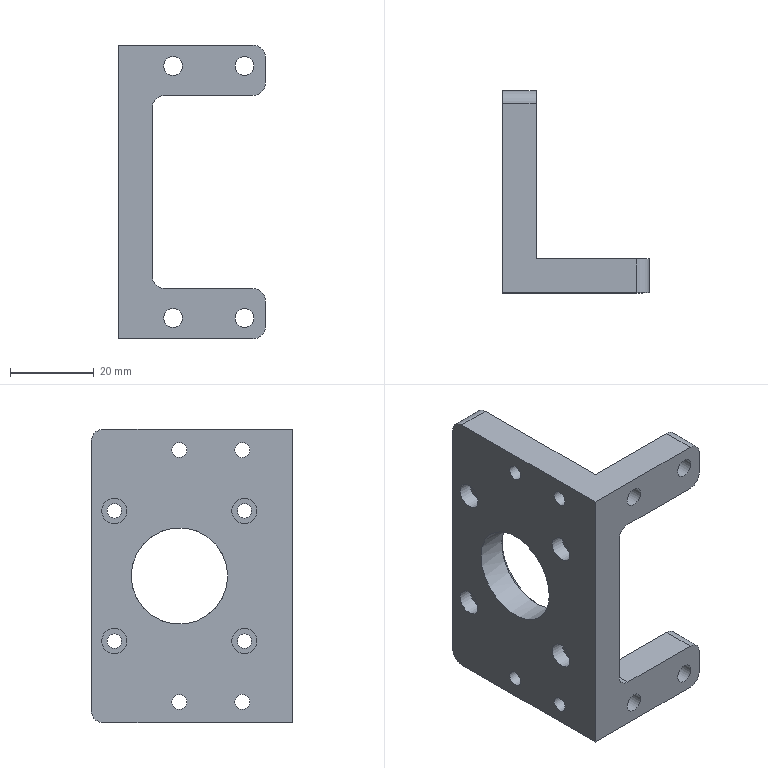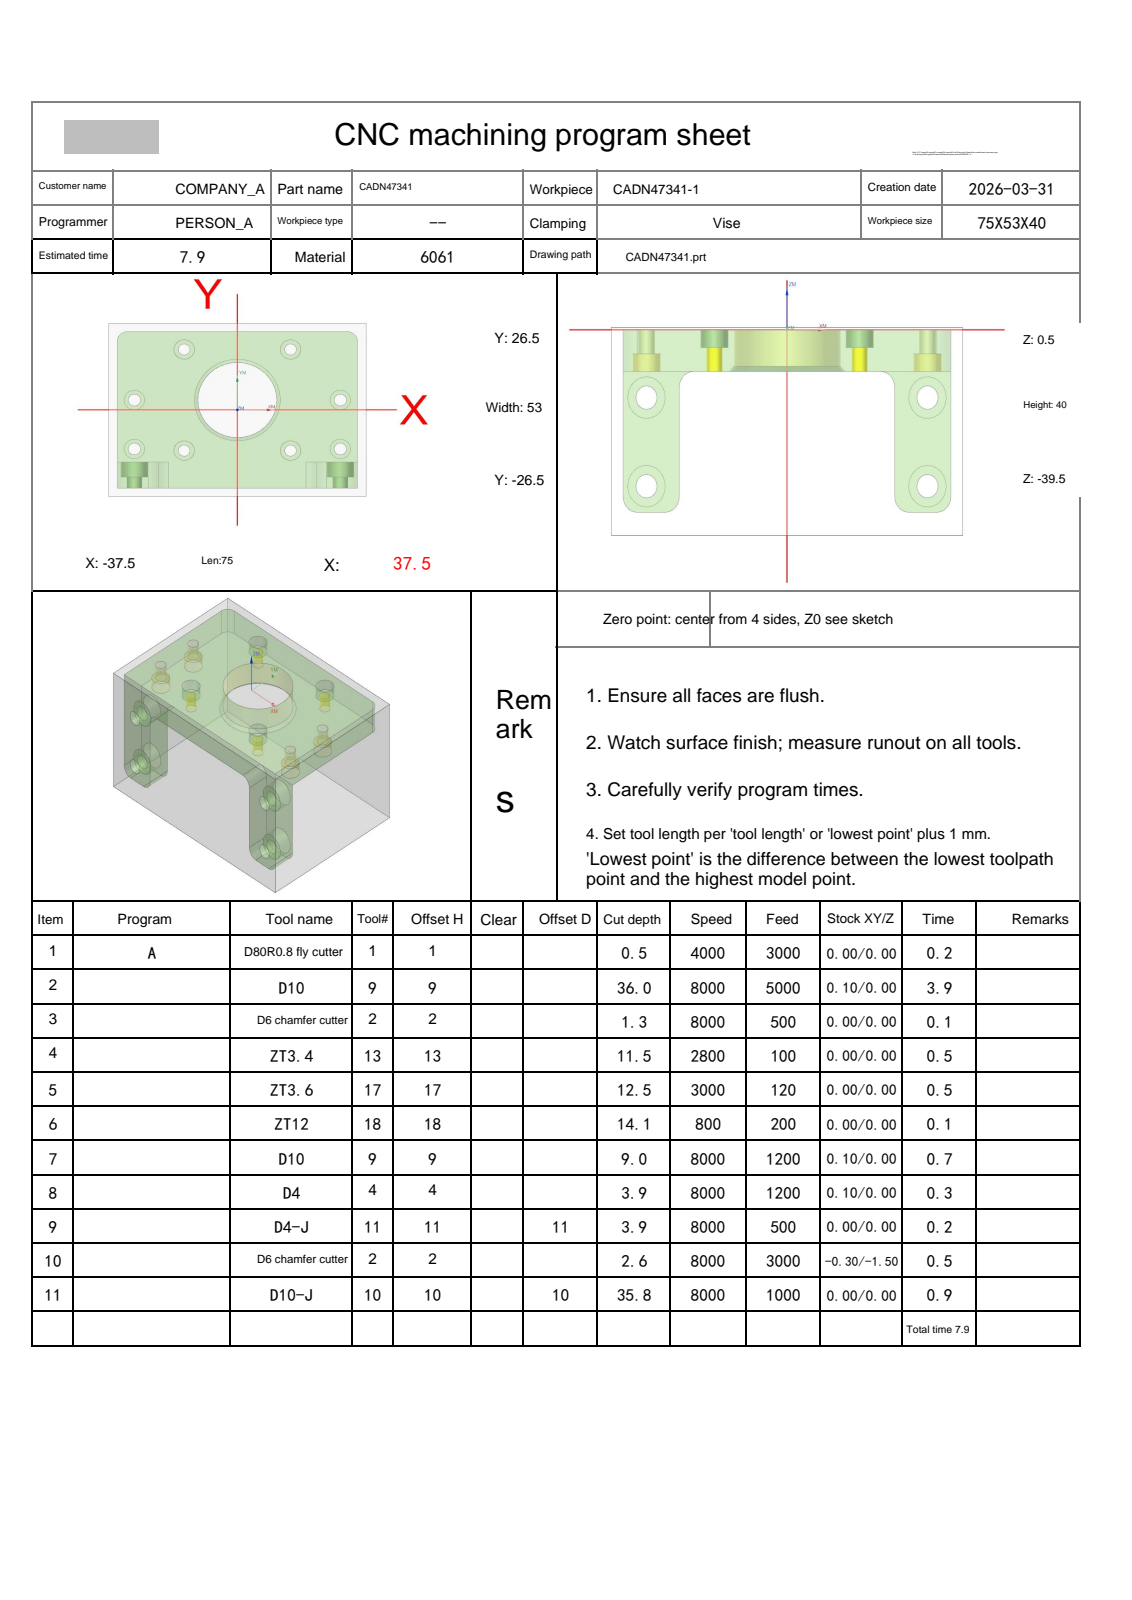NC program | NX | posted by the shop | part box 35 x 48 x 70 mm
Whole program:
%
O0001
(Machine time: 9.90 MIN)
(===Total Tool:9===)
(T1=D80R0.8 fly cutter D=80.  R=0.8  D-  H01 Z=0.    )
(T9=D10     D=10.  R=0.   D-  H09 Z=-35.5 )
(T2=D6 chamfer cutter   D=6.   R=0.   D-  H02 Z=-2.1  )
(T13=ZT3.4  D=3.4  DR_a=118 D-  H13 Z=-11.02)
(T17=ZT3.6  D=3.6  DR_a=118 D-  H17 Z=-12.  )
(T18=ZT12   D=12.  DR_a=118 D-  H18 Z=-13.61)
(T4=D4      D=4.   R=0.   D-  H04 Z=-3.4  )
(T11=D4-J   D=4.   R=0.   D11 H11 Z=-3.4  )
(T10=D10-J  D=10.  R=0.   D10 H10 Z=-35.3 )
G80 G90 G17 G49 G40
G91 G28 Z0
M01
N1 T01 M06
(D80R0.8 fly cutter  D=80. R=0.8 H=01 ce=0.20 di=0.10)
G00 G90 G54 X-80. Y0.0 M03 S4000
G43 H01 Z20.
M08
Z2.1
G01 Z.1 F3000.
X-75.
X75.
X80.
Z2.1
G00 Z20.
G00 G90 X-80. Y0.0 M03 S4000
Z20.
Z2.
G01 Z0.0 F1000.
X-75.
X75.
X80.
Z2.
G00 Z20.
G91 G28 Z0.0
M05
M09
G91 G28 Z0.0
M01
N2 T09 M06
(D10  D=10. R=0. H=09 ce=0.10 di=0.00)
G00 G90 G54 X0.0 Y-29.1 M03 S8000
G43 H09 Z20.
M08
Z.5
G01 X-35. Z.435 F5000.
G02 X-40.1 Y-24. Z.42 I0.0 J5.1
G01 Y21. Z.337
G02 X-32. Y29.1 Z.313 I8.1 J0.0
G01 X32. Z.194
G02 X40.1 Y21. Z.17 I0.0 J-8.1
G01 Y-24. Z.087
G02 X35. Y-29.1 Z.072 I-5.1 J0.0
G01 X-35. Z-.058
G02 X-40.1 Y-24. Z-.073 I0.0 J5.1
G01 Y21. Z-.157
G02 X-32. Y29.1 Z-.18 I8.1 J0.0
G01 X32. Z-.299
G02 X40.1 Y21. Z-.323 I0.0 J-8.1
G01 Y-24. Z-.406
G02 X35. Y-29.1 Z-.421 I-5.1 J0.0
G01 X-35. Z-.551
G02 X-40.1 Y-24. Z-.566 I0.0 J5.1
G01 Y21. Z-.65
G02 X-32. Y29.1 Z-.673 I8.1 J0.0
G01 X32. Z-.792
G02 X40.1 Y21. Z-.816 I0.0 J-8.1
G01 Y-24. Z-.9
G02 X35. Y-29.1 Z-.914 I-5.1 J0.0
G01 X-35. Z-1.044
G02 X-40.1 Y-24. Z-1.059 I0.0 J5.1
G01 Y21. Z-1.143
G02 X-32. Y29.1 Z-1.167 I8.1 J0.0
G01 X32. Z-1.285
G02 X40.1 Y21. Z-1.309 I0.0 J-8.1
G01 Y-24. Z-1.393
G02 X35. Y-29.1 Z-1.408 I-5.1 J0.0
G01 X-35. Z-1.538
G02 X-40.1 Y-24. Z-1.553 I0.0 J5.1
G01 Y21. Z-1.636
G02 X-32. Y29.1 Z-1.66 I8.1 J0.0
G01 X32. Z-1.779
G02 X40.1 Y21. Z-1.802 I0.0 J-8.1
G01 Y-24. Z-1.886
G02 X35. Y-29.1 Z-1.901 I-5.1 J0.0
G01 X-35. Z-2.031
G02 X-40.1 Y-24. Z-2.046 I0.0 J5.1
G01 Y21. Z-2.129
G02 X-32. Y29.1 Z-2.153 I8.1 J0.0
G01 X32. Z-2.272
G02 X40.1 Y21. Z-2.295 I0.0 J-8.1
G01 Y-24. Z-2.379
G02 X35. Y-29.1 Z-2.394 I-5.1 J0.0
G01 X-35. Z-2.524
G02 X-40.1 Y-24. Z-2.539 I0.0 J5.1
G01 Y21. Z-2.622
G02 X-32. Y29.1 Z-2.646 I8.1 J0.0
G01 X32. Z-2.765
G02 X40.1 Y21. Z-2.789 I0.0 J-8.1
G01 Y-24. Z-2.872
G02 X35. Y-29.1 Z-2.887 I-5.1 J0.0
G01 X-35. Z-3.017
G02 X-40.1 Y-24. Z-3.032 I0.0 J5.1
G01 Y21. Z-3.116
G02 X-32. Y29.1 Z-3.139 I8.1 J0.0
G01 X32. Z-3.258
G02 X40.1 Y21. Z-3.282 I0.0 J-8.1
G01 Y-24. Z-3.365
G02 X35. Y-29.1 Z-3.38 I-5.1 J0.0
G01 X-35. Z-3.51
G02 X-40.1 Y-24. Z-3.525 I0.0 J5.1
G01 Y21. Z-3.609
G02 X-32. Y29.1 Z-3.632 I8.1 J0.0
G01 X32. Z-3.751
G02 X40.1 Y21. Z-3.775 I0.0 J-8.1
G01 Y-24. Z-3.858
G02 X35. Y-29.1 Z-3.873 I-5.1 J0.0
G01 X-35. Z-4.003
G02 X-40.1 Y-24. Z-4.018 I0.0 J5.1
G01 Y21. Z-4.102
G02 X-32. Y29.1 Z-4.125 I8.1 J0.0
G01 X32. Z-4.244
G02 X40.1 Y21. Z-4.268 I0.0 J-8.1
G01 Y-24. Z-4.352
G02 X35. Y-29.1 Z-4.366 I-5.1 J0.0
G01 X-35. Z-4.497
G02 X-40.1 Y-24. Z-4.511 I0.0 J5.1
G01 Y21. Z-4.595
G02 X-32. Y29.1 Z-4.619 I8.1 J0.0
G01 X32. Z-4.738
G02 X40.1 Y21. Z-4.761 I0.0 J-8.1
G01 Y-24. Z-4.845
G02 X35. Y-29.1 Z-4.86 I-5.1 J0.0
G01 X-35. Z-4.99
G02 X-40.1 Y-24. Z-5.005 I0.0 J5.1
G01 Y21. Z-5.088
G02 X-32. Y29.1 Z-5.112 I8.1 J0.0
G01 X32. Z-5.231
G02 X40.1 Y21. Z-5.254 I0.0 J-8.1
G01 Y-24. Z-5.338
G02 X35. Y-29.1 Z-5.353 I-5.1 J0.0
G01 X-35. Z-5.483
G02 X-40.1 Y-24. Z-5.498 I0.0 J5.1
G01 Y21. Z-5.581
G02 X-32. Y29.1 Z-5.605 I8.1 J0.0
G01 X32. Z-5.724
G02 X40.1 Y21. Z-5.747 I0.0 J-8.1
G01 Y-24. Z-5.831
G02 X35. Y-29.1 Z-5.846 I-5.1 J0.0
G01 X-35. Z-5.976
G02 X-40.1 Y-24. Z-5.991 I0.0 J5.1
G01 Y21. Z-6.074
G02 X-32. Y29.1 Z-6.098 I8.1 J0.0
G01 X32. Z-6.217
G02 X40.1 Y21. Z-6.241 I0.0 J-8.1
G01 Y-24. Z-6.324
G02 X35. Y-29.1 Z-6.339 I-5.1 J0.0
G01 X-35. Z-6.469
G02 X-40.1 Y-24. Z-6.484 I0.0 J5.1
G01 Y21. Z-6.568
G02 X-32. Y29.1 Z-6.591 I8.1 J0.0
G01 X32. Z-6.71
G02 X40.1 Y21. Z-6.734 I0.0 J-8.1
G01 Y-24. Z-6.817
G02 X35. Y-29.1 Z-6.832 I-5.1 J0.0
G01 X-35. Z-6.962
G02 X-40.1 Y-24. Z-6.977 I0.0 J5.1
G01 Y21. Z-7.061
G02 X-32. Y29.1 Z-7.084 I8.1 J0.0
G01 X32. Z-7.203
G02 X40.1 Y21. Z-7.227 I0.0 J-8.1
G01 Y-24. Z-7.311
G02 X35. Y-29.1 Z-7.325 I-5.1 J0.0
G01 X-35. Z-7.455
G02 X-40.1 Y-24. Z-7.47 I0.0 J5.1
G01 Y21. Z-7.554
G02 X-32. Y29.1 Z-7.578 I8.1 J0.0
G01 X32. Z-7.696
G02 X40.1 Y21. Z-7.72 I0.0 J-8.1
G01 Y-24. Z-7.804
G02 X35. Y-29.1 Z-7.819 I-5.1 J0.0
G01 X-35. Z-7.949
G02 X-40.1 Y-24. Z-7.963 I0.0 J5.1
G01 Y21. Z-8.047
G02 X-32. Y29.1 Z-8.071 I8.1 J0.0
G01 X32. Z-8.19
G02 X40.1 Y21. Z-8.213 I0.0 J-8.1
G01 Y-24. Z-8.297
G02 X35. Y-29.1 Z-8.312 I-5.1 J0.0
G01 X-35. Z-8.442
G02 X-40.1 Y-24. Z-8.457 I0.0 J5.1
G01 Y21. Z-8.54
G02 X-32. Y29.1 Z-8.564 I8.1 J0.0
G01 X32. Z-8.683
G02 X40.1 Y21. Z-8.706 I0.0 J-8.1
G01 Y-24. Z-8.79
G02 X35. Y-29.1 Z-8.805 I-5.1 J0.0
G01 X-35. Z-8.935
G02 X-40.1 Y-24. Z-8.95 I0.0 J5.1
G01 Y21. Z-9.033
G02 X-32. Y29.1 Z-9.057 I8.1 J0.0
G01 X32. Z-9.176
G02 X40.1 Y21. Z-9.2 I0.0 J-8.1
G01 Y-24. Z-9.283
G02 X35. Y-29.1 Z-9.298 I-5.1 J0.0
G01 X-35. Z-9.428
G02 X-40.1 Y-24. Z-9.443 I0.0 J5.1
G01 Y21. Z-9.527
G02 X-32. Y29.1 Z-9.55 I8.1 J0.0
G01 X32. Z-9.669
G02 X40.1 Y21. Z-9.693 I0.0 J-8.1
G01 Y-24. Z-9.776
G02 X35. Y-29.1 Z-9.791 I-5.1 J0.0
G01 X-35. Z-9.921
G02 X-40.1 Y-24. Z-9.936 I0.0 J5.1
G01 Y21. Z-10.02
G02 X-32. Y29.1 Z-10.043 I8.1 J0.0
G01 X32. Z-10.162
G02 X40.1 Y21. Z-10.186 I0.0 J-8.1
G01 Y-24. Z-10.269
G02 X35. Y-29.1 Z-10.284 I-5.1 J0.0
G01 X-35. Z-10.414
G02 X-40.1 Y-24. Z-10.429 I0.0 J5.1
G01 Y21. Z-10.513
G02 X-32. Y29.1 Z-10.536 I8.1 J0.0
G01 X32. Z-10.655
G02 X40.1 Y21. Z-10.679 I0.0 J-8.1
G01 Y-24. Z-10.763
G02 X35. Y-29.1 Z-10.777 I-5.1 J0.0
G01 X-35. Z-10.907
G02 X-40.1 Y-24. Z-10.922 I0.0 J5.1
G01 Y21. Z-11.006
G02 X-32. Y29.1 Z-11.03 I8.1 J0.0
G01 X32. Z-11.148
G02 X40.1 Y21. Z-11.172 I0.0 J-8.1
G01 Y-24. Z-11.256
G02 X35. Y-29.1 Z-11.271 I-5.1 J0.0
G01 X-35. Z-11.401
G02 X-40.1 Y-24. Z-11.416 I0.0 J5.1
G01 Y21. Z-11.499
G02 X-32. Y29.1 Z-11.523 I8.1 J0.0
G01 X32. Z-11.642
G02 X40.1 Y21. Z-11.665 I0.0 J-8.1
G01 Y-24. Z-11.749
G02 X35. Y-29.1 Z-11.764 I-5.1 J0.0
G01 X-35. Z-11.894
G02 X-40.1 Y-24. Z-11.909 I0.0 J5.1
G01 Y21. Z-11.992
G02 X-32. Y29.1 Z-12.016 I8.1 J0.0
G01 X32. Z-12.135
G02 X40.1 Y21. Z-12.158 I0.0 J-8.1
G01 Y-24. Z-12.242
G02 X35. Y-29.1 Z-12.257 I-5.1 J0.0
G01 X-35. Z-12.387
G02 X-40.1 Y-24. Z-12.402 I0.0 J5.1
G01 Y21. Z-12.485
G02 X-32. Y29.1 Z-12.509 I8.1 J0.0
G01 X32. Z-12.628
G02 X40.1 Y21. Z-12.652 I0.0 J-8.1
G01 Y-24. Z-12.735
G02 X35. Y-29.1 Z-12.75 I-5.1 J0.0
G01 X-35. Z-12.88
G02 X-40.1 Y-24. Z-12.895 I0.0 J5.1
G01 Y21. Z-12.979
G02 X-32. Y29.1 Z-13.002 I8.1 J0.0
G01 X32. Z-13.121
G02 X40.1 Y21. Z-13.145 I0.0 J-8.1
G01 Y-24. Z-13.228
G02 X35. Y-29.1 Z-13.243 I-5.1 J0.0
G01 X-35. Z-13.373
G02 X-40.1 Y-24. Z-13.388 I0.0 J5.1
G01 Y21. Z-13.472
G02 X-32. Y29.1 Z-13.495 I8.1 J0.0
G01 X32. Z-13.614
G02 X40.1 Y21. Z-13.638 I0.0 J-8.1
G01 Y-24. Z-13.721
G02 X35. Y-29.1 Z-13.736 I-5.1 J0.0
G01 X-35. Z-13.866
G02 X-40.1 Y-24. Z-13.881 I0.0 J5.1
G01 Y21. Z-13.965
G02 X-32. Y29.1 Z-13.989 I8.1 J0.0
G01 X32. Z-14.107
G02 X40.1 Y21. Z-14.131 I0.0 J-8.1
G01 Y-24. Z-14.215
G02 X35. Y-29.1 Z-14.23 I-5.1 J0.0
G01 X-35. Z-14.36
G02 X-40.1 Y-24. Z-14.374 I0.0 J5.1
G01 Y21. Z-14.458
G02 X-32. Y29.1 Z-14.482 I8.1 J0.0
G01 X32. Z-14.601
G02 X40.1 Y21. Z-14.624 I0.0 J-8.1
G01 Y-24. Z-14.708
G02 X35. Y-29.1 Z-14.723 I-5.1 J0.0
G01 X-35. Z-14.853
G02 X-40.1 Y-24. Z-14.868 I0.0 J5.1
G01 Y21. Z-14.951
G02 X-32. Y29.1 Z-14.975 I8.1 J0.0
G01 X32. Z-15.094
G02 X40.1 Y21. Z-15.117 I0.0 J-8.1
G01 Y-24. Z-15.201
G02 X35. Y-29.1 Z-15.216 I-5.1 J0.0
G01 X-35. Z-15.346
G02 X-40.1 Y-24. Z-15.361 I0.0 J5.1
G01 Y21. Z-15.444
G02 X-32. Y29.1 Z-15.468 I8.1 J0.0
G01 X32. Z-15.587
G02 X40.1 Y21. Z-15.61 I0.0 J-8.1
G01 Y-24. Z-15.694
G02 X35. Y-29.1 Z-15.709 I-5.1 J0.0
G01 X-35. Z-15.839
G02 X-40.1 Y-24. Z-15.854 I0.0 J5.1
G01 Y21. Z-15.937
G02 X-32. Y29.1 Z-15.961 I8.1 J0.0
G01 X32. Z-16.08
G02 X40.1 Y21. Z-16.104 I0.0 J-8.1
G01 Y-24. Z-16.187
G02 X35. Y-29.1 Z-16.202 I-5.1 J0.0
G01 X-35. Z-16.332
G02 X-40.1 Y-24. Z-16.347 I0.0 J5.1
G01 Y21. Z-16.431
G02 X-32. Y29.1 Z-16.454 I8.1 J0.0
G01 X32. Z-16.573
G02 X40.1 Y21. Z-16.597 I0.0 J-8.1
G01 Y-24. Z-16.68
G02 X35. Y-29.1 Z-16.695 I-5.1 J0.0
G01 X-35. Z-16.825
G02 X-40.1 Y-24. Z-16.84 I0.0 J5.1
G01 Y21. Z-16.924
G02 X-32. Y29.1 Z-16.947 I8.1 J0.0
G01 X32. Z-17.066
G02 X40.1 Y21. Z-17.09 I0.0 J-8.1
G01 Y-24. Z-17.174
G02 X35. Y-29.1 Z-17.188 I-5.1 J0.0
G01 X-35. Z-17.318
G02 X-40.1 Y-24. Z-17.333 I0.0 J5.1
G01 Y21. Z-17.417
G02 X-32. Y29.1 Z-17.441 I8.1 J0.0
G01 X32. Z-17.559
G02 X40.1 Y21. Z-17.583 I0.0 J-8.1
G01 Y-24. Z-17.667
G02 X35. Y-29.1 Z-17.682 I-5.1 J0.0
G01 X-35. Z-17.812
G02 X-40.1 Y-24. Z-17.826 I0.0 J5.1
G01 Y21. Z-17.91
G02 X-32. Y29.1 Z-17.934 I8.1 J0.0
G01 X32. Z-18.053
G02 X40.1 Y21. Z-18.076 I0.0 J-8.1
G01 Y-24. Z-18.16
G02 X35. Y-29.1 Z-18.175 I-5.1 J0.0
G01 X-35. Z-18.305
G02 X-40.1 Y-24. Z-18.32 I0.0 J5.1
G01 Y21. Z-18.403
G02 X-32. Y29.1 Z-18.427 I8.1 J0.0
G01 X32. Z-18.546
G02 X40.1 Y21. Z-18.569 I0.0 J-8.1
G01 Y-24. Z-18.653
G02 X35. Y-29.1 Z-18.668 I-5.1 J0.0
G01 X-35. Z-18.798
G02 X-40.1 Y-24. Z-18.813 I0.0 J5.1
G01 Y21. Z-18.896
G02 X-32. Y29.1 Z-18.92 I8.1 J0.0
G01 X32. Z-19.039
G02 X40.1 Y21. Z-19.063 I0.0 J-8.1
G01 Y-24. Z-19.146
G02 X35. Y-29.1 Z-19.161 I-5.1 J0.0
G01 X-35. Z-19.291
G02 X-40.1 Y-24. Z-19.306 I0.0 J5.1
G01 Y21. Z-19.39
G02 X-32. Y29.1 Z-19.413 I8.1 J0.0
G01 X32. Z-19.532
G02 X40.1 Y21. Z-19.556 I0.0 J-8.1
G01 Y-24. Z-19.639
G02 X35. Y-29.1 Z-19.654 I-5.1 J0.0
G01 X-35. Z-19.784
G02 X-40.1 Y-24. Z-19.799 I0.0 J5.1
G01 Y21. Z-19.883
G02 X-32. Y29.1 Z-19.906 I8.1 J0.0
G01 X32. Z-20.025
G02 X40.1 Y21. Z-20.049 I0.0 J-8.1
G01 Y-24. Z-20.132
G02 X35. Y-29.1 Z-20.147 I-5.1 J0.0
G01 X-35. Z-20.277
G02 X-40.1 Y-24. Z-20.292 I0.0 J5.1
G01 Y21. Z-20.376
G02 X-32. Y29.1 Z-20.399 I8.1 J0.0
G01 X32. Z-20.518
G02 X40.1 Y21. Z-20.542 I0.0 J-8.1
G01 Y-24. Z-20.626
G02 X35. Y-29.1 Z-20.64 I-5.1 J0.0
G01 X-35. Z-20.77
G02 X-40.1 Y-24. Z-20.785 I0.0 J5.1
G01 Y21. Z-20.869
G02 X-32. Y29.1 Z-20.893 I8.1 J0.0
G01 X32. Z-21.012
G02 X40.1 Y21. Z-21.035 I0.0 J-8.1
G01 Y-24. Z-21.119
G02 X35. Y-29.1 Z-21.134 I-5.1 J0.0
G01 X-35. Z-21.264
G02 X-40.1 Y-24. Z-21.279 I0.0 J5.1
G01 Y21. Z-21.362
G02 X-32. Y29.1 Z-21.386 I8.1 J0.0
G01 X32. Z-21.505
G02 X40.1 Y21. Z-21.528 I0.0 J-8.1
G01 Y-24. Z-21.612
G02 X35. Y-29.1 Z-21.627 I-5.1 J0.0
G01 X-35. Z-21.757
G02 X-40.1 Y-24. Z-21.772 I0.0 J5.1
G01 Y21. Z-21.855
G02 X-32. Y29.1 Z-21.879 I8.1 J0.0
G01 X32. Z-21.998
G02 X40.1 Y21. Z-22.021 I0.0 J-8.1
G01 Y-24. Z-22.105
G02 X35. Y-29.1 Z-22.12 I-5.1 J0.0
G01 X-35. Z-22.25
G02 X-40.1 Y-24. Z-22.265 I0.0 J5.1
G01 Y21. Z-22.348
G02 X-32. Y29.1 Z-22.372 I8.1 J0.0
G01 X32. Z-22.491
G02 X40.1 Y21. Z-22.515 I0.0 J-8.1
G01 Y-24. Z-22.598
G02 X35. Y-29.1 Z-22.613 I-5.1 J0.0
G01 X-35. Z-22.743
G02 X-40.1 Y-24. Z-22.758 I0.0 J5.1
G01 Y21. Z-22.842
G02 X-32. Y29.1 Z-22.865 I8.1 J0.0
G01 X32. Z-22.984
G02 X40.1 Y21. Z-23.008 I0.0 J-8.1
G01 Y-24. Z-23.091
G02 X35. Y-29.1 Z-23.106 I-5.1 J0.0
G01 X-35. Z-23.236
G02 X-40.1 Y-24. Z-23.251 I0.0 J5.1
G01 Y21. Z-23.335
G02 X-32. Y29.1 Z-23.358 I8.1 J0.0
G01 X32. Z-23.477
G02 X40.1 Y21. Z-23.501 I0.0 J-8.1
G01 Y-24. Z-23.584
G02 X35. Y-29.1 Z-23.599 I-5.1 J0.0
G01 X-35. Z-23.729
G02 X-40.1 Y-24. Z-23.744 I0.0 J5.1
G01 Y21. Z-23.828
G02 X-32. Y29.1 Z-23.852 I8.1 J0.0
G01 X32. Z-23.97
G02 X40.1 Y21. Z-23.994 I0.0 J-8.1
G01 Y-24. Z-24.078
G02 X35. Y-29.1 Z-24.093 I-5.1 J0.0
G01 X-35. Z-24.223
G02 X-40.1 Y-24. Z-24.237 I0.0 J5.1
G01 Y21. Z-24.321
G02 X-32. Y29.1 Z-24.345 I8.1 J0.0
G01 X32. Z-24.464
G02 X40.1 Y21. Z-24.487 I0.0 J-8.1
G01 Y-24. Z-24.571
G02 X35. Y-29.1 Z-24.586 I-5.1 J0.0
G01 X-35. Z-24.716
G02 X-40.1 Y-24. Z-24.731 I0.0 J5.1
G01 Y21. Z-24.814
G02 X-32. Y29.1 Z-24.838 I8.1 J0.0
G01 X32. Z-24.957
G02 X40.1 Y21. Z-24.98 I0.0 J-8.1
G01 Y-24. Z-25.064
G02 X35. Y-29.1 Z-25.079 I-5.1 J0.0
G01 X-35. Z-25.209
G02 X-40.1 Y-24. Z-25.224 I0.0 J5.1
G01 Y21. Z-25.307
G02 X-32. Y29.1 Z-25.331 I8.1 J0.0
G01 X32. Z-25.45
G02 X40.1 Y21. Z-25.473 I0.0 J-8.1
G01 Y-24. Z-25.557
G02 X35. Y-29.1 Z-25.572 I-5.1 J0.0
G01 X-35. Z-25.702
G02 X-40.1 Y-24. Z-25.717 I0.0 J5.1
G01 Y21. Z-25.8
G02 X-32. Y29.1 Z-25.824 I8.1 J0.0
G01 X32. Z-25.943
G02 X40.1 Y21. Z-25.967 I0.0 J-8.1
G01 Y-24. Z-26.05
G02 X35. Y-29.1 Z-26.065 I-5.1 J0.0
G01 X-35. Z-26.195
G02 X-40.1 Y-24. Z-26.21 I0.0 J5.1
G01 Y21. Z-26.294
G02 X-32. Y29.1 Z-26.317 I8.1 J0.0
G01 X32. Z-26.436
G02 X40.1 Y21. Z-26.46 I0.0 J-8.1
G01 Y-24. Z-26.543
G02 X35. Y-29.1 Z-26.558 I-5.1 J0.0
G01 X-35. Z-26.688
G02 X-40.1 Y-24. Z-26.703 I0.0 J5.1
G01 Y21. Z-26.787
G02 X-32. Y29.1 Z-26.81 I8.1 J0.0
G01 X32. Z-26.929
G02 X40.1 Y21. Z-26.953 I0.0 J-8.1
G01 Y-24. Z-27.037
G02 X35. Y-29.1 Z-27.051 I-5.1 J0.0
G01 X-35. Z-27.181
G02 X-40.1 Y-24. Z-27.196 I0.0 J5.1
G01 Y21. Z-27.28
G02 X-32. Y29.1 Z-27.304 I8.1 J0.0
G01 X32. Z-27.422
G02 X40.1 Y21. Z-27.446 I0.0 J-8.1
G01 Y-24. Z-27.53
G02 X35. Y-29.1 Z-27.545 I-5.1 J0.0
G01 X-35. Z-27.675
G02 X-40.1 Y-24. Z-27.689 I0.0 J5.1
G01 Y21. Z-27.773
G02 X-32. Y29.1 Z-27.797 I8.1 J0.0
G01 X32. Z-27.916
G02 X40.1 Y21. Z-27.939 I0.0 J-8.1
G01 Y-24. Z-28.023
G02 X35. Y-29.1 Z-28.038 I-5.1 J0.0
G01 X-35. Z-28.168
G02 X-40.1 Y-24. Z-28.183 I0.0 J5.1
G01 Y21. Z-28.266
G02 X-32. Y29.1 Z-28.29 I8.1 J0.0
G01 X32. Z-28.409
G02 X40.1 Y21. Z-28.432 I0.0 J-8.1
G01 Y-24. Z-28.516
G02 X35. Y-29.1 Z-28.531 I-5.1 J0.0
G01 X-35. Z-28.661
G02 X-40.1 Y-24. Z-28.676 I0.0 J5.1
G01 Y21. Z-28.759
G02 X-32. Y29.1 Z-28.783 I8.1 J0.0
G01 X32. Z-28.902
G02 X40.1 Y21. Z-28.926 I0.0 J-8.1
G01 Y-24. Z-29.009
G02 X35. Y-29.1 Z-29.024 I-5.1 J0.0
G01 X-35. Z-29.154
G02 X-40.1 Y-24. Z-29.169 I0.0 J5.1
G01 Y21. Z-29.253
G02 X-32. Y29.1 Z-29.276 I8.1 J0.0
G01 X32. Z-29.395
G02 X40.1 Y21. Z-29.419 I0.0 J-8.1
G01 Y-24. Z-29.502
G02 X35. Y-29.1 Z-29.517 I-5.1 J0.0
G01 X-35. Z-29.647
G02 X-40.1 Y-24. Z-29.662 I0.0 J5.1
G01 Y21. Z-29.746
G02 X-32. Y29.1 Z-29.769 I8.1 J0.0
G01 X32. Z-29.888
G02 X40.1 Y21. Z-29.912 I0.0 J-8.1
G01 Y-24. Z-29.995
G02 X35. Y-29.1 Z-30.01 I-5.1 J0.0
G01 X-35. Z-30.14
G02 X-40.1 Y-24. Z-30.155 I0.0 J5.1
G01 Y21. Z-30.239
G02 X-32. Y29.1 Z-30.262 I8.1 J0.0
G01 X32. Z-30.381
G02 X40.1 Y21. Z-30.405 I0.0 J-8.1
G01 Y-24. Z-30.489
G02 X35. Y-29.1 Z-30.503 I-5.1 J0.0
G01 X-35. Z-30.634
G02 X-40.1 Y-24. Z-30.648 I0.0 J5.1
G01 Y21. Z-30.732
G02 X-32. Y29.1 Z-30.756 I8.1 J0.0
G01 X32. Z-30.875
G02 X40.1 Y21. Z-30.898 I0.0 J-8.1
G01 Y-24. Z-30.982
G02 X35. Y-29.1 Z-30.997 I-5.1 J0.0
G01 X-35. Z-31.127
G02 X-40.1 Y-24. Z-31.142 I0.0 J5.1
G01 Y21. Z-31.225
G02 X-32. Y29.1 Z-31.249 I8.1 J0.0
G01 X32. Z-31.368
G02 X40.1 Y21. Z-31.391 I0.0 J-8.1
G01 Y-24. Z-31.475
G02 X35. Y-29.1 Z-31.49 I-5.1 J0.0
G01 X-35. Z-31.62
G02 X-40.1 Y-24. Z-31.635 I0.0 J5.1
G01 Y21. Z-31.718
G02 X-32. Y29.1 Z-31.742 I8.1 J0.0
G01 X32. Z-31.861
G02 X40.1 Y21. Z-31.884 I0.0 J-8.1
G01 Y-24. Z-31.968
G02 X35. Y-29.1 Z-31.983 I-5.1 J0.0
G01 X-35. Z-32.113
G02 X-40.1 Y-24. Z-32.128 I0.0 J5.1
G01 Y21. Z-32.211
G02 X-32. Y29.1 Z-32.235 I8.1 J0.0
G01 X32. Z-32.354
G02 X40.1 Y21. Z-32.378 I0.0 J-8.1
G01 Y-24. Z-32.461
G02 X35. Y-29.1 Z-32.476 I-5.1 J0.0
G01 X-35. Z-32.606
G02 X-40.1 Y-24. Z-32.621 I0.0 J5.1
G01 Y21. Z-32.705
G02 X-32. Y29.1 Z-32.728 I8.1 J0.0
G01 X32. Z-32.847
G02 X40.1 Y21. Z-32.871 I0.0 J-8.1
G01 Y-24. Z-32.954
G02 X35. Y-29.1 Z-32.969 I-5.1 J0.0
G01 X-35. Z-33.099
G02 X-40.1 Y-24. Z-33.114 I0.0 J5.1
G01 Y21. Z-33.198
G02 X-32. Y29.1 Z-33.221 I8.1 J0.0
G01 X32. Z-33.34
G02 X40.1 Y21. Z-33.364 I0.0 J-8.1
G01 Y-24. Z-33.447
G02 X35. Y-29.1 Z-33.462 I-5.1 J0.0
G01 X-35. Z-33.592
G02 X-40.1 Y-24. Z-33.607 I0.0 J5.1
G01 Y21. Z-33.691
G02 X-32. Y29.1 Z-33.715 I8.1 J0.0
G01 X32. Z-33.833
G02 X40.1 Y21. Z-33.857 I0.0 J-8.1
G01 Y-24. Z-33.941
G02 X35. Y-29.1 Z-33.956 I-5.1 J0.0
G01 X-35. Z-34.086
G02 X-40.1 Y-24. Z-34.1 I0.0 J5.1
G01 Y21. Z-34.184
G02 X-32. Y29.1 Z-34.208 I8.1 J0.0
G01 X32. Z-34.327
G02 X40.1 Y21. Z-34.35 I0.0 J-8.1
G01 Y-24. Z-34.434
G02 X35. Y-29.1 Z-34.449 I-5.1 J0.0
G01 X-35. Z-34.579
G02 X-40.1 Y-24. Z-34.594 I0.0 J5.1
G01 Y21. Z-34.677
G02 X-32. Y29.1 Z-34.701 I8.1 J0.0
G01 X32. Z-34.82
G02 X40.1 Y21. Z-34.843 I0.0 J-8.1
G01 Y-24. Z-34.927
G02 X35. Y-29.1 Z-34.942 I-5.1 J0.0
G01 X-35. Z-35.072
G02 X-40.1 Y-24. Z-35.087 I0.0 J5.1
G01 Y21. Z-35.17
G02 X-32. Y29.1 Z-35.194 I8.1 J0.0
G01 X32. Z-35.313
G02 X40.1 Y21. Z-35.337 I0.0 J-8.1
G01 Y-24. Z-35.42
G02 X35. Y-29.1 Z-35.435 I-5.1 J0.0
G01 X0.0 Z-35.5
X-35.
G02 X-40.1 Y-24. I0.0 J5.1
G01 Y21.
G02 X-32. Y29.1 I8.1 J0.0
G01 X32.
G02 X40.1 Y21. I0.0 J-8.1
G01 Y-24.
G02 X35. Y-29.1 I-5.1 J0.0
G01 X0.0
X-.5
Z-34.5
G00 Z20.
G91 G28 Z0.0
M05
M09
G91 G28 Z0.0
M01
N3 T02 M06
(D6 chamfer cutter  D=6. R=0. H=02 ce=0.00 di=0.00)
G00 G90 G54 X15.5 Y18.5 M03 S8000
G43 H02 Z20.
M08
G98 G81 X15.5 Y18.5 Z-.8 R1. F500.
X30. Y3.
Y-12.
X15.5 Y-12.5
X0.0 Y3.
X-15.5 Y18.5
X-30. Y3.
Y-12.
X-15.5 Y-12.5
G80
G00 Z20.
G91 G28 Z0.0
M05
M09
G91 G28 Z0.0
M01
N4 T13 M06
(ZT3.4 D=3.4 DR_a=118 H=13)
G00 G90 G54 X15.5 Y-12.5 M03 S2800
G43 H13 Z20.
M08
G98 G83 X15.5 Y-12.5 Z-11.021 R1. F100. Q2.
X-15.5
Y18.5
X15.5
G80
G00 Z20.
G91 G28 Z0.0
M05
M09
G91 G28 Z0.0
M01
N5 T17 M06
(ZT3.6 D=3.6 DR_a=118 H=17)
G00 G90 G54 X-30. Y3. M03 S3000
G43 H17 Z20.
M08
G98 G83 X-30. Y3. Z-12. R1. F120. Q3.
Y-12.
X30.
Y3.
G80
G00 Z20.
G91 G28 Z0.0
M05
M09
G91 G28 Z0.0
M01
N6 T18 M06
(ZT12 D=12. DR_a=118 H=18)
G00 G90 G54 X0.0 Y3. M03 S800
G43 H18 Z20.
M08
G98 G83 X0.0 Y3. Z-13.605 R1. F200. Q3.
G80
G00 Z20.
G91 G28 Z0.0
M05
M09
G91 G28 Z0.0
M01
N7 T09 M06
(D10  D=10. R=0. H=09 ce=0.10 di=0.00)
G00 G90 G54 X0.0 Y3. M03 S8000
G43 H09 Z20.
M08
Z.5
G03 X3.2 Y6.2 I0.0 J3.2 F1200.
X0.0 Y9.4 I-3.2 J0.0
X0.0 Y9.4 Z0.0 I0.0 J-6.4
X0.0 Y9.4 Z-.5 I0.0 J-6.4
X0.0 Y9.4 Z-1. I0.0 J-6.4
X0.0 Y9.4 Z-1.5 I0.0 J-6.4
X0.0 Y9.4 Z-2. I0.0 J-6.4
X0.0 Y9.4 Z-2.5 I0.0 J-6.4
X0.0 Y9.4 Z-3. I0.0 J-6.4
X0.0 Y9.4 Z-3.5 I0.0 J-6.4
X0.0 Y9.4 Z-4. I0.0 J-6.4
X0.0 Y9.4 Z-4.5 I0.0 J-6.4
X0.0 Y9.4 Z-5. I0.0 J-6.4
X0.0 Y9.4 Z-5.5 I0.0 J-6.4
X0.0 Y9.4 Z-6. I0.0 J-6.4
X0.0 Y9.4 Z-6.5 I0.0 J-6.4
X0.0 Y9.4 Z-7. I0.0 J-6.4
X0.0 Y9.4 Z-7.5 I0.0 J-6.4
X0.0 Y9.4 Z-8. I0.0 J-6.4
X0.0 Y9.4 Z-8.5 I0.0 J-6.4
X-6.4 Y3. I0.0 J-6.4
X0.0 Y-3.4 I6.4 J0.0
X6.4 Y3. I0.0 J6.4
X0.0 Y9.4 I-6.4 J0.0
X-3.2 Y6.2 I0.0 J-3.2
X0.0 Y3. I3.2 J0.0
G00 Z20.
G91 G28 Z0.0
M05
M09
G91 G28 Z0.0
M01
N8 T04 M06
(D4  D=4. R=0. H=04 ce=0.10 di=0.00)
G00 G90 G54 X15.5 Y-12.5 M03 S8000
G43 H04 Z20.
M08
Z.5
G03 X15.95 Y-12.05 I0.0 J.45 F1200.
X15.5 Y-11.6 I-.45 J0.0
X15.5 Y-11.6 Z.2 I0.0 J-.9
X15.5 Y-11.6 Z-.1 I0.0 J-.9
X15.5 Y-11.6 Z-.4 I0.0 J-.9
X15.5 Y-11.6 Z-.7 I0.0 J-.9
X15.5 Y-11.6 Z-1. I0.0 J-.9
X15.5 Y-11.6 Z-1.3 I0.0 J-.9
X15.5 Y-11.6 Z-1.6 I0.0 J-.9
X15.5 Y-11.6 Z-1.9 I0.0 J-.9
X15.5 Y-11.6 Z-2.2 I0.0 J-.9
X15.5 Y-11.6 Z-2.5 I0.0 J-.9
X15.5 Y-11.6 Z-2.8 I0.0 J-.9
X15.5 Y-11.6 Z-3.1 I0.0 J-.9
X15.5 Y-11.6 Z-3.4 I0.0 J-.9
X14.6 Y-12.5 I0.0 J-.9
X15.5 Y-13.4 I.9 J0.0
X16.4 Y-12.5 I0.0 J.9
X15.5 Y-11.6 I-.9 J0.0
X15.05 Y-12.05 I0.0 J-.45
X15.5 Y-12.5 I.45 J0.0
G00 Z20.
X-15.5
Z.5
G03 X-15.05 Y-12.05 I0.0 J.45
X-15.5 Y-11.6 I-.45 J0.0
X-15.5 Y-11.6 Z.2 I0.0 J-.9
X-15.5 Y-11.6 Z-.1 I0.0 J-.9
X-15.5 Y-11.6 Z-.4 I0.0 J-.9
X-15.5 Y-11.6 Z-.7 I0.0 J-.9
X-15.5 Y-11.6 Z-1. I0.0 J-.9
X-15.5 Y-11.6 Z-1.3 I0.0 J-.9
X-15.5 Y-11.6 Z-1.6 I0.0 J-.9
X-15.5 Y-11.6 Z-1.9 I0.0 J-.9
X-15.5 Y-11.6 Z-2.2 I0.0 J-.9
X-15.5 Y-11.6 Z-2.5 I0.0 J-.9
X-15.5 Y-11.6 Z-2.8 I0.0 J-.9
X-15.5 Y-11.6 Z-3.1 I0.0 J-.9
X-15.5 Y-11.6 Z-3.4 I0.0 J-.9
X-16.4 Y-12.5 I0.0 J-.9
X-15.5 Y-13.4 I.9 J0.0
X-14.6 Y-12.5 I0.0 J.9
X-15.5 Y-11.6 I-.9 J0.0
X-15.95 Y-12.05 I0.0 J-.45
X-15.5 Y-12.5 I.45 J0.0
G00 Z20.
Y18.5
Z.5
G03 X-15.05 Y18.95 I0.0 J.45
X-15.5 Y19.4 I-.45 J0.0
X-15.5 Y19.4 Z.2 I0.0 J-.9
X-15.5 Y19.4 Z-.1 I0.0 J-.9
X-15.5 Y19.4 Z-.4 I0.0 J-.9
X-15.5 Y19.4 Z-.7 I0.0 J-.9
X-15.5 Y19.4 Z-1. I0.0 J-.9
X-15.5 Y19.4 Z-1.3 I0.0 J-.9
X-15.5 Y19.4 Z-1.6 I0.0 J-.9
X-15.5 Y19.4 Z-1.9 I0.0 J-.9
X-15.5 Y19.4 Z-2.2 I0.0 J-.9
X-15.5 Y19.4 Z-2.5 I0.0 J-.9
X-15.5 Y19.4 Z-2.8 I0.0 J-.9
X-15.5 Y19.4 Z-3.1 I0.0 J-.9
X-15.5 Y19.4 Z-3.4 I0.0 J-.9
X-16.4 Y18.5 I0.0 J-.9
X-15.5 Y17.6 I.9 J0.0
X-14.6 Y18.5 I0.0 J.9
X-15.5 Y19.4 I-.9 J0.0
X-15.95 Y18.95 I0.0 J-.45
X-15.5 Y18.5 I.45 J0.0
G00 Z20.
X15.5
Z.5
G03 X15.95 Y18.95 I0.0 J.45
X15.5 Y19.4 I-.45 J0.0
X15.5 Y19.4 Z.2 I0.0 J-.9
X15.5 Y19.4 Z-.1 I0.0 J-.9
X15.5 Y19.4 Z-.4 I0.0 J-.9
X15.5 Y19.4 Z-.7 I0.0 J-.9
X15.5 Y19.4 Z-1. I0.0 J-.9
X15.5 Y19.4 Z-1.3 I0.0 J-.9
X15.5 Y19.4 Z-1.6 I0.0 J-.9
X15.5 Y19.4 Z-1.9 I0.0 J-.9
X15.5 Y19.4 Z-2.2 I0.0 J-.9
X15.5 Y19.4 Z-2.5 I0.0 J-.9
X15.5 Y19.4 Z-2.8 I0.0 J-.9
X15.5 Y19.4 Z-3.1 I0.0 J-.9
X15.5 Y19.4 Z-3.4 I0.0 J-.9
X14.6 Y18.5 I0.0 J-.9
X15.5 Y17.6 I.9 J0.0
X16.4 Y18.5 I0.0 J.9
X15.5 Y19.4 I-.9 J0.0
X15.05 Y18.95 I0.0 J-.45
X15.5 Y18.5 I.45 J0.0
G00 Z20.
G91 G28 Z0.0
M05
M09
G91 G28 Z0.0
M01
N9 T11 M06
(D4-J  D=4. R=0. H=11 ce=0.00 di=0.00)
G00 G90 G54 X15.5 Y-12.5 M03 S8000
G43 H11 Z20.
M08
Z.5
G41 D11
G01 X15.685 Y-12.423 F500.
G03 X15.98 Y-11.98 I-.185 J.443
X15.5 Y-11.5 I-.48 J0.0
X16.482 Y-12.313 Z-3.4 I0.0 J-1.
X15.5 Y-11.5 I-.982 J-.187
X14.5 Y-12.5 I0.0 J-1.
X15.5 Y-13.5 I1. J0.0
X16.5 Y-12.5 I0.0 J1.
G01 X16.482 Y-12.313
G03 X16.011 Y-11.923 I-.471 J-.09
X15.541 Y-12.304 I0.0 J-.48
G01 G40 X15.5 Y-12.5
G00 Z20.
X-15.5
Z.5
G41 D11
G01 X-15.315 Y-12.423
G03 X-15.02 Y-11.98 I-.185 J.443
X-15.5 Y-11.5 I-.48 J0.0
X-14.518 Y-12.313 Z-3.4 I0.0 J-1.
X-15.5 Y-11.5 I-.982 J-.187
X-16.5 Y-12.5 I0.0 J-1.
X-15.5 Y-13.5 I1. J0.0
X-14.5 Y-12.5 I0.0 J1.
G01 X-14.518 Y-12.313
G03 X-14.989 Y-11.923 I-.471 J-.09
X-15.459 Y-12.304 I0.0 J-.48
G01 G40 X-15.5 Y-12.5
G00 Z20.
Y18.5
Z.5
G41 D11
G01 X-15.315 Y18.577
G03 X-15.02 Y19.02 I-.185 J.443
X-15.5 Y19.5 I-.48 J0.0
X-14.518 Y18.687 Z-3.4 I0.0 J-1.
X-15.5 Y19.5 I-.982 J-.187
X-16.5 Y18.5 I0.0 J-1.
X-15.5 Y17.5 I1. J0.0
X-14.5 Y18.5 I0.0 J1.
G01 X-14.518 Y18.687
G03 X-14.989 Y19.077 I-.471 J-.09
X-15.459 Y18.696 I0.0 J-.48
G01 G40 X-15.5 Y18.5
G00 Z20.
X15.5
Z.5
G41 D11
G01 X15.685 Y18.577
G03 X15.98 Y19.02 I-.185 J.443
X15.5 Y19.5 I-.48 J0.0
X16.482 Y18.687 Z-3.4 I0.0 J-1.
X15.5 Y19.5 I-.982 J-.187
X14.5 Y18.5 I0.0 J-1.
X15.5 Y17.5 I1. J0.0
X16.5 Y18.5 I0.0 J1.
G01 X16.482 Y18.687
G03 X16.011 Y19.077 I-.471 J-.09
X15.541 Y18.696 I0.0 J-.48
G01 G40 X15.5 Y18.5
G00 Z20.
G91 G28 Z0.0
M05
M09
G91 G28 Z0.0
M01
N10 T02 M06
(D6 chamfer cutter  D=6. R=0. H=02 ce=0.00 di=0.00)
G00 G90 G54 X.25 Y-26.128 M03 S8000
G43 H02 Z20.
M08
Z2.099
G01 Z-1.5 F3000.
G03 X.33 Y-25.828 I-.52 J.3
X.03 Y-25.308 I-.6 J0.0
G01 X0.0 Y-25.3
X-35.
G02 X-36.3 Y-24. I0.0 J1.3
G01 Y21.
G02 X-32. Y25.3 I4.3 J0.0
G01 X32.
G02 X36.3 Y21. I0.0 J-4.3
G01 Y-24.
G02 X35. Y-25.3 I-1.3 J0.0
G01 X0.0
X-.03 Y-25.308
G03 X-.33 Y-25.828 I.3 J-.52
X-.25 Y-26.128 I.6 J0.0
G01 Z2.099
G00 Z20.
X-9.384 Y3.285
Z2.125
G01 Z-1.5
G03 X-9.661 Y3.353 I-.277 J-.532
X-10.193 Y3.03 I0.0 J-.6
G01 X-10.2 Y3.
G03 X0.0 Y-7.2 I10.2 J0.0
X10.2 Y3. I0.0 J10.2
X0.0 Y13.2 I-10.2 J0.0
X-10.2 Y3. I0.0 J-10.2
G01 X-10.193 Y2.97
G03 X-9.661 Y2.647 I.532 J.277
X-9.384 Y2.715 I0.0 J.6
G01 Z2.125
G00 Z20.
G00 G90 X-30. Y3. M03 S8000
Z20.
G98 G81 X-30. Y3. Z-2.1 R3. F500.
Y-12.
X30.
Y3.
G80
G00 Z20.
G00 G90 X14.33 Y-10.519 M03 S8000
Z20.
Z2.5
G01 X14.248 Y-10.567 Z2.465 F500.
X13.987 Y-10.764 Z2.346
X13.756 Y-10.996 Z2.227
X13.56 Y-11.259 Z2.108
X13.404 Y-11.546 Z1.989
X13.29 Y-11.853 Z1.87
X13.22 Y-12.173 Z1.75
X13.197 Y-12.5 Z1.631
X13.22 Y-12.827 Z1.512
X13.29 Y-13.147 Z1.393
X13.404 Y-13.454 Z1.274
X13.56 Y-13.741 Z1.154
X13.756 Y-14.004 Z1.035
X13.987 Y-14.236 Z.916
X14.248 Y-14.433 Z.797
X14.452 Y-14.551 Z.711
X14.753 Y-14.679 Z.592
X15.07 Y-14.762 Z.473
X15.395 Y-14.801 Z.354
X15.722 Y-14.792 Z.235
X16.045 Y-14.738 Z.115
X16.357 Y-14.638 Z-.004
X16.652 Y-14.494 Z-.123
X16.923 Y-14.311 Z-.242
X17.165 Y-14.091 Z-.361
X17.374 Y-13.839 Z-.48
X17.545 Y-13.559 Z-.6
X17.674 Y-13.259 Z-.719
X17.76 Y-12.943 Z-.838
X17.8 Y-12.618 Z-.957
Y-12.5 Z-1.
G03 X15.5 Y-10.2 I-2.3 J0.0
X13.2 Y-12.5 I0.0 J-2.3
X15.5 Y-14.8 I2.3 J0.0
X17.8 Y-12.5 I0.0 J2.3
X17.746 Y-12.004 I-2.3 J0.0
G01 Z1.5
G00 Z20.
X-16.67 Y-10.519
Z2.5
G01 X-16.752 Y-10.567 Z2.465
X-17.013 Y-10.764 Z2.346
X-17.244 Y-10.996 Z2.227
X-17.44 Y-11.259 Z2.108
X-17.596 Y-11.546 Z1.989
X-17.71 Y-11.853 Z1.87
X-17.78 Y-12.173 Z1.75
X-17.803 Y-12.5 Z1.631
X-17.78 Y-12.827 Z1.512
X-17.71 Y-13.147 Z1.393
X-17.596 Y-13.454 Z1.274
X-17.44 Y-13.741 Z1.154
X-17.244 Y-14.004 Z1.035
X-17.013 Y-14.236 Z.916
X-16.752 Y-14.433 Z.797
X-16.548 Y-14.551 Z.711
X-16.247 Y-14.679 Z.592
X-15.93 Y-14.762 Z.473
X-15.605 Y-14.801 Z.354
X-15.278 Y-14.792 Z.235
X-14.955 Y-14.738 Z.115
X-14.643 Y-14.638 Z-.004
X-14.349 Y-14.494 Z-.123
X-14.077 Y-14.311 Z-.242
X-13.835 Y-14.091 Z-.361
X-13.626 Y-13.839 Z-.48
X-13.455 Y-13.559 Z-.6
X-13.326 Y-13.259 Z-.719
X-13.24 Y-12.943 Z-.838
X-13.2 Y-12.618 Z-.957
Y-12.5 Z-1.
G03 X-15.5 Y-10.2 I-2.3 J0.0
X-17.8 Y-12.5 I0.0 J-2.3
X-15.5 Y-14.8 I2.3 J0.0
X-13.2 Y-12.5 I0.0 J2.3
X-13.254 Y-12.004 I-2.3 J0.0
G01 Z1.5
G00 Z20.
X-16.67 Y20.481
Z2.5
G01 X-16.752 Y20.433 Z2.465
X-17.013 Y20.236 Z2.346
X-17.244 Y20.004 Z2.227
X-17.44 Y19.741 Z2.108
X-17.596 Y19.454 Z1.989
X-17.71 Y19.147 Z1.87
X-17.78 Y18.827 Z1.75
X-17.803 Y18.5 Z1.631
X-17.78 Y18.173 Z1.512
X-17.71 Y17.853 Z1.393
X-17.596 Y17.546 Z1.274
X-17.44 Y17.259 Z1.154
X-17.244 Y16.996 Z1.035
X-17.013 Y16.764 Z.916
X-16.752 Y16.567 Z.797
X-16.548 Y16.449 Z.711
X-16.247 Y16.321 Z.592
X-15.93 Y16.238 Z.473
X-15.605 Y16.199 Z.354
X-15.278 Y16.208 Z.235
X-14.955 Y16.262 Z.115
X-14.643 Y16.362 Z-.004
X-14.349 Y16.506 Z-.123
X-14.077 Y16.689 Z-.242
X-13.835 Y16.909 Z-.361
X-13.626 Y17.161 Z-.48
X-13.455 Y17.441 Z-.6
X-13.326 Y17.741 Z-.719
X-13.24 Y18.057 Z-.838
X-13.2 Y18.382 Z-.957
Y18.5 Z-1.
G03 X-15.5 Y20.8 I-2.3 J0.0
X-17.8 Y18.5 I0.0 J-2.3
X-15.5 Y16.2 I2.3 J0.0
X-13.2 Y18.5 I0.0 J2.3
X-13.254 Y18.996 I-2.3 J0.0
G01 Z1.5
G00 Z20.
X14.33 Y20.481
Z2.5
G01 X14.248 Y20.433 Z2.465
X13.987 Y20.236 Z2.346
X13.756 Y20.004 Z2.227
X13.56 Y19.741 Z2.108
X13.404 Y19.454 Z1.989
X13.29 Y19.147 Z1.87
X13.22 Y18.827 Z1.75
X13.197 Y18.5 Z1.631
X13.22 Y18.173 Z1.512
X13.29 Y17.853 Z1.393
X13.404 Y17.546 Z1.274
X13.56 Y17.259 Z1.154
X13.756 Y16.996 Z1.035
X13.987 Y16.764 Z.916
X14.248 Y16.567 Z.797
X14.452 Y16.449 Z.711
X14.753 Y16.321 Z.592
X15.07 Y16.238 Z.473
X15.395 Y16.199 Z.354
X15.722 Y16.208 Z.235
X16.045 Y16.262 Z.115
X16.357 Y16.362 Z-.004
X16.652 Y16.506 Z-.123
X16.923 Y16.689 Z-.242
X17.165 Y16.909 Z-.361
X17.374 Y17.161 Z-.48
X17.545 Y17.441 Z-.6
X17.674 Y17.741 Z-.719
X17.76 Y18.057 Z-.838
X17.8 Y18.382 Z-.957
Y18.5 Z-1.
G03 X15.5 Y20.8 I-2.3 J0.0
X13.2 Y18.5 I0.0 J-2.3
X15.5 Y16.2 I2.3 J0.0
X17.8 Y18.5 I0.0 J2.3
X17.746 Y18.996 I-2.3 J0.0
G01 Z1.5
G00 Z20.
G00 G90 X-7.3 Y6. M03 S8000
Z20.
Z-1.
G01 Z-1.5 F1000.
G03 X-10.3 Y3. I0.0 J-3.
X0.0 Y-7.3 I10.3 J0.0
X10.3 Y3. I0.0 J10.3
X0.0 Y13.3 I-10.3 J0.0
X-10.3 Y3. I0.0 J-10.3
X-7.3 Y0.0 I3. J0.0
G01 Z-1.
G00 Z20.
G91 G28 Z0.0
M05
M09
G91 G28 Z0.0
M01
N11 T10 M06
(D10-J  D=10. R=0. H=10 ce=0.00 di=0.00)
G00 G90 G54 X36.013 Y-30.116 M03 S8000
G43 H10 Z20.
M08
Z-11.267
G01 Z-11.767 F1000.
G41 D10
X35.997 Y-29.917
G03 X35. Y-29. I-.997 J-.083
G01 X-35.
G02 X-40. Y-24. I0.0 J5.
G01 Y21.
G02 X-32. Y29. I8. J0.0
G01 X32.
G02 X40. Y21. I0.0 J-8.
G01 Y-24.
G02 X35. Y-29. I-5. J0.0
G01 X34.5
G03 X33.5 Y-30. I0.0 J-1.
G01 G40 Y-30.2
Z-11.267
G00 Z20.
X36.013 Y-30.116
Z-23.033
G01 Z-23.533
G41 D10
X35.997 Y-29.917
G03 X35. Y-29. I-.997 J-.083
G01 X-35.
G02 X-40. Y-24. I0.0 J5.
G01 Y21.
G02 X-32. Y29. I8. J0.0
G01 X32.
G02 X40. Y21. I0.0 J-8.
G01 Y-24.
G02 X35. Y-29. I-5. J0.0
G01 X34.5
G03 X33.5 Y-30. I0.0 J-1.
G01 G40 Y-30.2
Z-23.033
G00 Z20.
X36.013 Y-30.116
Z-34.8
G01 Z-35.3
G41 D10
X35.997 Y-29.917
G03 X35. Y-29. I-.997 J-.083
G01 X-35.
G02 X-40. Y-24. I0.0 J5.
G01 Y21.
G02 X-32. Y29. I8. J0.0
G01 X32.
G02 X40. Y21. I0.0 J-8.
G01 Y-24.
G02 X35. Y-29. I-5. J0.0
G01 X34.5
G03 X33.5 Y-30. I0.0 J-1.
G01 G40 Y-30.2
Z-34.8
G00 Z20.
G00 G90 X1.5 Y7.57 M03 S8000
Z10.5
Z-5.7
G01 Z-7.2 F1000.
G41 D10
Y8.
G03 X0.0 Y9.5 I-1.5 J0.0
X-6.5 Y3. I0.0 J-6.5
X0.0 Y-3.5 I6.5 J0.0
X6.5 Y3. I0.0 J6.5
X0.0 Y9.5 I-6.5 J0.0
X-.4 Y9.488 I0.0 J-6.5
X-1.807 Y7.991 I.092 J-1.497
G01 X-1.805 Y7.898
X-1.79 Y7.668
G40 X-1.778 Y7.469
Z-5.7
G00 Z10.5
M05
M09
G91 G28 Z0.0
G91 G28 Y0.0
M30
%